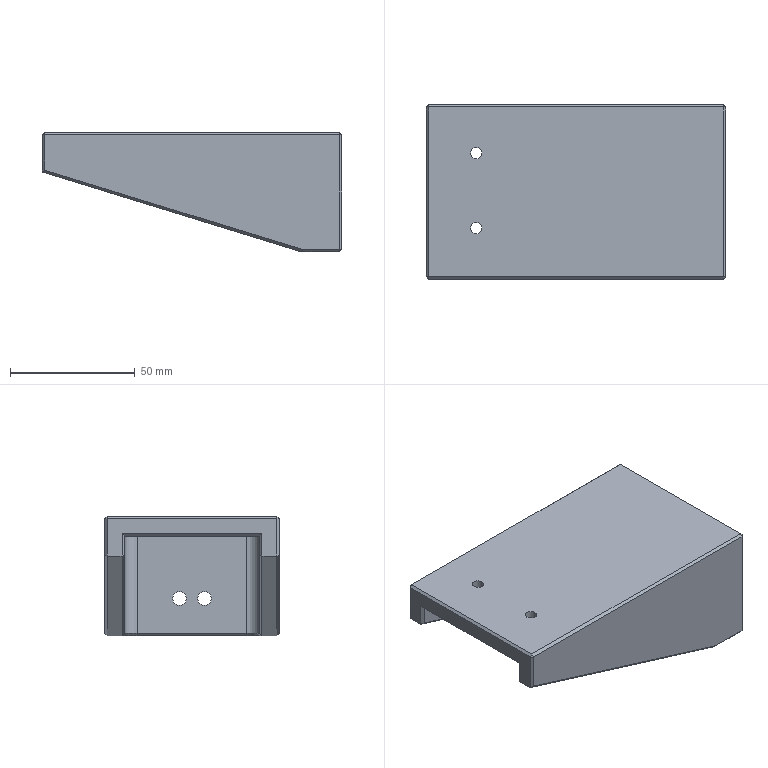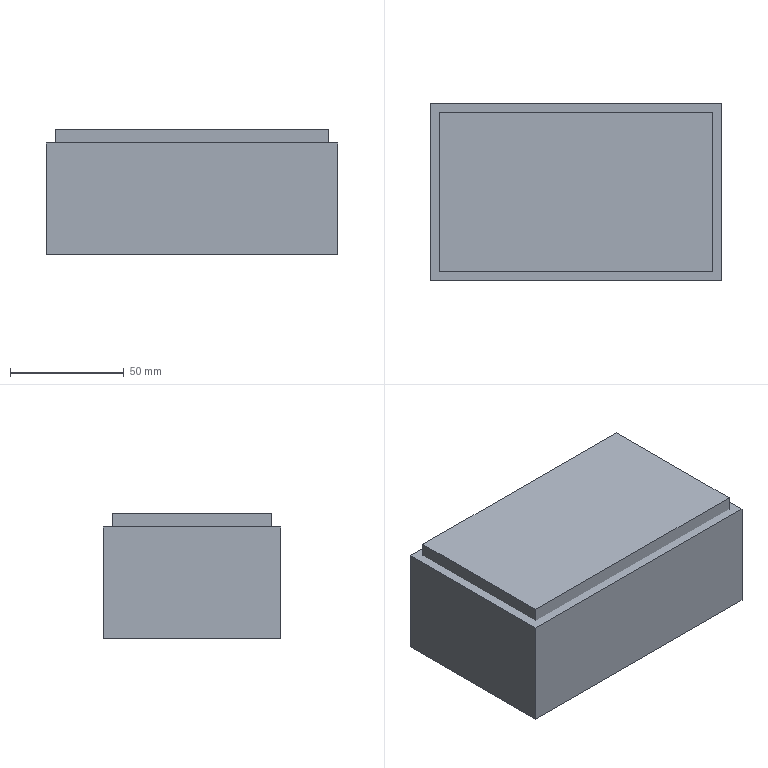CAM job | NX | 3+2 milling, drilling | part box 120 x 70 x 48 mm | stock box 128 x 78 x 55 mm
Tools:
number,name,description,diameter,corner_radius,flute_length,length,flutes
1,D63,Milling Tool-5 Parameters,63.0,0.0,50.0,75.0,2
9,D6A45,Milling Tool-5 Parameters,6.0,0.0,3.0,3.0,2
14,4.5ZT,Drilling Tool,4.5,0.0,35.0,50.0,2
2,D10,Milling Tool-5 Parameters,10.0,0.0,50.0,75.0,2
17,5.5ZT,Drilling Tool,5.5,0.0,35.0,50.0,2
18,D6R0.5,Milling Tool-5 Parameters,6.0,0.5,50.0,75.0,2
Operations:
program,operation,operation_type,tool,method,geometry_group,spindle_rpm,surface_speed,feed_per_tooth,feed_cut,feed_plunge,cut_length_mm,path_length_mm,cut_time_min,machine_time_min
1-125-75-55毛胚,FLOOR_WALL,VolumeBased25DMillingOperation,D63,METHOD,A,6500.0,0.0,0.0,1250.0,100.0,637.797,691.797,0.5102,0.5156
1-125-75-55毛胚,DRILLING,Operation,D6A45,METHOD,A,4000.0,75.0,0.0312,250.0,0.0,8.0,109.15,0.032,0.0421
1-125-75-55毛胚,DRILLING_COPY,Operation,4.5ZT,METHOD,A,2000.0,20.0,0.05,200.0,0.0,27.704,148.557,0.1385,0.1506
1-125-75-55毛胚,ZLEVEL_PROFILE_COPY_COPY_COPY_1,ZLevelMilling,D10,METHOD,A,7000.0,351.0,0.1429,2000.0,1000.0,22343.589,22499.589,11.246,11.261
1-125-75-55毛胚,ZLEVEL_PROFILE_COPY,ZLevelMilling,D10,METHOD,A,6500.0,326.0,0.0769,1000.0,1000.0,1254.218,1408.214,1.254,1.27
1-125-75-55毛胚,ZLEVEL_PROFILE_COPY_1_COPY_COPY_COPY_COPY_COPY_COPY,ZLevelMilling,D6A45,METHOD,A,7000.0,131.0,0.0714,1000.0,1000.0,398.504,644.055,0.3985,0.4231
2-125-75-55毛胚,DRILLING_COPY_1,Operation,D6A45,METHOD,B,4000.0,75.0,0.0312,250.0,0.0,11.7,96.84,0.0468,0.0553
2-125-75-55毛胚,DRILLING_COPY_COPY,Operation,5.5ZT,METHOD,B,2000.0,20.0,0.05,200.0,0.0,28.305,130.05,0.1415,0.1517
3-125-75-55毛胚,FLOOR_WALL_COPY,VolumeBased25DMillingOperation,D63,METHOD,C,6500.0,0.0,0.0,1250.0,100.0,2959.579,3564.363,2.368,2.428
3-125-75-55毛胚,ADAPTIVE_MILLING,CavityMilling,D10,METHOD,C,7000.0,219.0,0.1429,2000.0,1000.0,39783.668,47461.019,19.994,20.762
3-125-75-55毛胚,FLOOR_WALL_1_COPY_COPY,VolumeBased25DMillingOperation,D10,METHOD,C,7000.0,219.0,0.0714,1000.0,1000.0,1429.008,1575.967,1.429,1.444
3-125-75-55毛胚,FLOOR_WALL_1_COPY_COPY_COPY,VolumeBased25DMillingOperation,D10,METHOD,C,7000.0,219.0,0.0714,1000.0,1000.0,549.351,779.44,0.5494,0.5757
3-125-75-55毛胚,ZLEVEL_PROFILE_1,ZLevelMilling,D6R0.5,METHOD,C,7000.0,131.0,0.1786,2500.0,1000.0,50961.981,51783.037,20.396,20.478
3-125-75-55毛胚,ZLEVEL_PROFILE_COPY_1_COPY_COPY_COPY_COPY_COPY_COPY_COPY,ZLevelMilling,D6A45,METHOD,C,7000.0,131.0,0.0714,1000.0,1000.0,177.228,313.445,0.1772,0.1908
3-125-75-55毛胚,ZLEVEL_PROFILE_COPY_1_COPY_COPY_COPY_COPY_COPY_COPY_COPY_COPY,ZLevelMilling,D6A45,METHOD,C,7000.0,131.0,0.0714,1000.0,1000.0,65.291,545.19,0.0653,0.1133